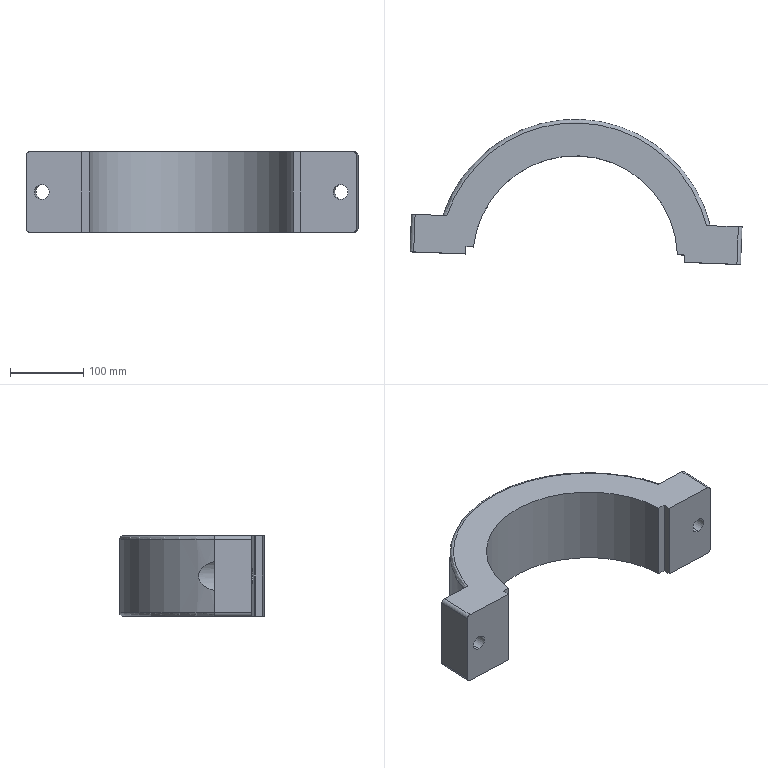Part | SolidWorks | features BaseBody 1 | 1 solid | 26 faces | box 454.449 x 198.703 x 110 mm | volume 3221578 mm3 | plane 12 | cylinder 12 | torus 2 | commonest cylinder face diameters 10 x4 20 x4 60 x2 280 x1 380 x1
STEP:
#1=CARTESIAN_POINT('',(121.261,1068.497,205.107));
#2=VERTEX_POINT('',#1);
#3=CARTESIAN_POINT('',(121.261,1068.497,315.107));
#4=VERTEX_POINT('',#3);
#5=CARTESIAN_POINT('',(121.261,1068.497,315.107));
#6=DIRECTION('',(0.,0.,1.));
#7=VECTOR('',#6,1000.);
#8=LINE('',#5,#7);
#9=EDGE_CURVE('',#2,#4,#8,.T.);
#10=ORIENTED_EDGE('',*,*,#9,.T.);
#11=CARTESIAN_POINT('',(110.911,1068.895,315.107));
#12=VERTEX_POINT('',#11);
#13=CARTESIAN_POINT('',(260.936,1063.128,315.107));
#14=DIRECTION('',(-0.9993,0.03842,0.));
#15=VECTOR('',#14,1000.);
#16=LINE('',#13,#15);
#17=EDGE_CURVE('',#4,#12,#16,.T.);
#18=ORIENTED_EDGE('',*,*,#17,.T.);
#19=CARTESIAN_POINT('',(110.911,1068.895,205.107));
#20=VERTEX_POINT('',#19);
#21=CARTESIAN_POINT('',(110.911,1068.895,-875.938));
#22=DIRECTION('',(0.,0.,1.));
#23=VECTOR('',#22,1000.);
#24=LINE('',#21,#23);
#25=EDGE_CURVE('',#20,#12,#24,.T.);
#26=ORIENTED_EDGE('',*,*,#25,.F.);
#27=CARTESIAN_POINT('',(260.936,1063.128,205.107));
#28=DIRECTION('',(-0.9993,0.03842,0.));
#29=VECTOR('',#28,1000.);
#30=LINE('',#27,#29);
#31=EDGE_CURVE('',#2,#20,#30,.T.);
#32=ORIENTED_EDGE('',*,*,#31,.F.);
#33=EDGE_LOOP('',(#10,#18,#26,#32));
#34=FACE_OUTER_BOUND('',#33,.T.);
#35=CARTESIAN_POINT('',(410.689,1057.37,-875.938));
#36=DIRECTION('',(0.03842,0.9993,0.));
#37=DIRECTION('',(0.,0.,-1.));
#38=AXIS2_PLACEMENT_3D('',#35,#36,#37);
#39=PLANE('',#38);
#40=ADVANCED_FACE('',(#34),#39,.F.);
#41=CARTESIAN_POINT('',(55.968,1061.,270.107));
#42=VERTEX_POINT('',#41);
#43=CARTESIAN_POINT('',(55.968,1061.,250.107));
#44=VERTEX_POINT('',#43);
#45=CARTESIAN_POINT('',(55.968,1061.,260.107));
#46=DIRECTION('',(-0.03842,-0.9993,0.));
#47=DIRECTION('',(0.,0.,1.));
#48=AXIS2_PLACEMENT_3D('',#45,#46,#47);
#49=CIRCLE('',#48,10.);
#50=EDGE_CURVE('',#42,#44,#49,.T.);
#51=ORIENTED_EDGE('',*,*,#50,.F.);
#52=CARTESIAN_POINT('',(55.968,1061.,260.107));
#53=DIRECTION('',(-0.03842,-0.9993,0.));
#54=DIRECTION('',(0.,0.,1.));
#55=AXIS2_PLACEMENT_3D('',#52,#53,#54);
#56=CIRCLE('',#55,10.);
#57=EDGE_CURVE('',#44,#42,#56,.T.);
#58=ORIENTED_EDGE('',*,*,#57,.F.);
#59=EDGE_LOOP('',(#51,#58));
#60=FACE_BOUND('',#59,.T.);
#61=CARTESIAN_POINT('',(110.527,1058.903,205.107));
#62=VERTEX_POINT('',#61);
#63=CARTESIAN_POINT('',(110.527,1058.903,315.107));
#64=VERTEX_POINT('',#63);
#65=CARTESIAN_POINT('',(110.527,1058.903,-875.938));
#66=DIRECTION('',(0.,0.,1.));
#67=VECTOR('',#66,1000.);
#68=LINE('',#65,#67);
#69=EDGE_CURVE('',#62,#64,#68,.T.);
#70=ORIENTED_EDGE('',*,*,#69,.T.);
#71=CARTESIAN_POINT('',(39.31,1061.641,315.107));
#72=VERTEX_POINT('',#71);
#73=CARTESIAN_POINT('',(260.552,1053.135,315.107));
#74=DIRECTION('',(-0.9993,0.03842,0.));
#75=VECTOR('',#74,1000.);
#76=LINE('',#73,#75);
#77=EDGE_CURVE('',#64,#72,#76,.T.);
#78=ORIENTED_EDGE('',*,*,#77,.T.);
#79=CARTESIAN_POINT('',(34.314,1061.833,310.107));
#80=VERTEX_POINT('',#79);
#81=CARTESIAN_POINT('',(39.31,1061.641,310.107));
#82=DIRECTION('',(-0.03842,-0.9993,0.));
#83=DIRECTION('',(0.,0.,1.));
#84=AXIS2_PLACEMENT_3D('',#81,#82,#83);
#85=CIRCLE('',#84,5.);
#86=EDGE_CURVE('',#72,#80,#85,.T.);
#87=ORIENTED_EDGE('',*,*,#86,.T.);
#88=CARTESIAN_POINT('',(34.314,1061.833,210.107));
#89=VERTEX_POINT('',#88);
#90=CARTESIAN_POINT('',(34.314,1061.833,315.107));
#91=DIRECTION('',(0.,0.,1.));
#92=VECTOR('',#91,1000.);
#93=LINE('',#90,#92);
#94=EDGE_CURVE('',#89,#80,#93,.T.);
#95=ORIENTED_EDGE('',*,*,#94,.F.);
#96=CARTESIAN_POINT('',(39.31,1061.641,205.107));
#97=VERTEX_POINT('',#96);
#98=CARTESIAN_POINT('',(39.31,1061.641,210.107));
#99=DIRECTION('',(-0.03842,-0.9993,0.));
#100=DIRECTION('',(0.,0.,1.));
#101=AXIS2_PLACEMENT_3D('',#98,#99,#100);
#102=CIRCLE('',#101,5.);
#103=EDGE_CURVE('',#89,#97,#102,.T.);
#104=ORIENTED_EDGE('',*,*,#103,.T.);
#105=CARTESIAN_POINT('',(260.552,1053.135,205.107));
#106=DIRECTION('',(-0.9993,0.03842,0.));
#107=VECTOR('',#106,1000.);
#108=LINE('',#105,#107);
#109=EDGE_CURVE('',#62,#97,#108,.T.);
#110=ORIENTED_EDGE('',*,*,#109,.F.);
#111=EDGE_LOOP('',(#70,#78,#87,#95,#104,#110));
#112=FACE_OUTER_BOUND('',#111,.T.);
#113=CARTESIAN_POINT('',(110.527,1058.903,-875.938));
#114=DIRECTION('',(0.03842,0.9993,0.));
#115=DIRECTION('',(0.,0.,-1.));
#116=AXIS2_PLACEMENT_3D('',#113,#114,#115);
#117=PLANE('',#116);
#118=ADVANCED_FACE('',(#60,#112),#117,.F.);
#119=ORIENTED_EDGE('',*,*,#25,.T.);
#120=CARTESIAN_POINT('',(79.906,262.409,315.107));
#121=DIRECTION('',(-0.03842,-0.9993,0.));
#122=VECTOR('',#121,1000.);
#123=LINE('',#120,#122);
#124=EDGE_CURVE('',#12,#64,#123,.T.);
#125=ORIENTED_EDGE('',*,*,#124,.T.);
#126=ORIENTED_EDGE('',*,*,#69,.F.);
#127=CARTESIAN_POINT('',(79.906,262.409,205.107));
#128=DIRECTION('',(-0.03842,-0.9993,0.));
#129=VECTOR('',#128,1000.);
#130=LINE('',#127,#129);
#131=EDGE_CURVE('',#20,#62,#130,.T.);
#132=ORIENTED_EDGE('',*,*,#131,.F.);
#133=EDGE_LOOP('',(#119,#125,#126,#132));
#134=FACE_OUTER_BOUND('',#133,.T.);
#135=CARTESIAN_POINT('',(110.911,1068.895,-875.938));
#136=DIRECTION('',(-0.9993,0.03842,0.));
#137=DIRECTION('',(0.,0.,1.));
#138=AXIS2_PLACEMENT_3D('',#135,#136,#137);
#139=PLANE('',#138);
#140=ADVANCED_FACE('',(#134),#139,.F.);
#141=CARTESIAN_POINT('',(481.794,1044.629,205.107));
#142=VERTEX_POINT('',#141);
#143=CARTESIAN_POINT('',(486.791,1044.437,210.107));
#144=VERTEX_POINT('',#143);
#145=CARTESIAN_POINT('',(481.794,1044.629,210.107));
#146=DIRECTION('',(-0.03842,-0.9993,0.));
#147=DIRECTION('',(0.,0.,1.));
#148=AXIS2_PLACEMENT_3D('',#145,#146,#147);
#149=CIRCLE('',#148,5.);
#150=EDGE_CURVE('',#142,#144,#149,.T.);
#151=ORIENTED_EDGE('',*,*,#150,.F.);
#152=CARTESIAN_POINT('',(483.767,1095.943,205.107));
#153=VERTEX_POINT('',#152);
#154=CARTESIAN_POINT('',(479.822,993.316,205.107));
#155=DIRECTION('',(-0.03842,-0.9993,0.));
#156=VECTOR('',#155,1000.);
#157=LINE('',#154,#156);
#158=EDGE_CURVE('',#153,#142,#157,.T.);
#159=ORIENTED_EDGE('',*,*,#158,.F.);
#160=CARTESIAN_POINT('',(488.763,1095.751,210.107));
#161=VERTEX_POINT('',#160);
#162=CARTESIAN_POINT('',(483.767,1095.943,210.107));
#163=DIRECTION('',(0.03842,0.9993,0.));
#164=DIRECTION('',(0.,0.,-1.));
#165=AXIS2_PLACEMENT_3D('',#162,#163,#164);
#166=CIRCLE('',#165,5.);
#167=EDGE_CURVE('',#161,#153,#166,.T.);
#168=ORIENTED_EDGE('',*,*,#167,.F.);
#169=CARTESIAN_POINT('',(488.763,1095.751,210.107));
#170=DIRECTION('',(0.03842,0.9993,0.));
#171=VECTOR('',#170,1000.);
#172=LINE('',#169,#171);
#173=EDGE_CURVE('',#144,#161,#172,.T.);
#174=ORIENTED_EDGE('',*,*,#173,.F.);
#175=EDGE_LOOP('',(#151,#159,#168,#174));
#176=FACE_OUTER_BOUND('',#175,.T.);
#177=CARTESIAN_POINT('',(451.173,248.135,210.107));
#178=DIRECTION('',(0.03842,0.9993,0.));
#179=DIRECTION('',(0.,0.,-1.));
#180=AXIS2_PLACEMENT_3D('',#177,#178,#179);
#181=CYLINDRICAL_SURFACE('',#180,5.);
#182=ADVANCED_FACE('',(#176),#181,.T.);
#183=ORIENTED_EDGE('',*,*,#103,.F.);
#184=CARTESIAN_POINT('',(36.287,1113.146,210.107));
#185=VERTEX_POINT('',#184);
#186=CARTESIAN_POINT('',(3.693,265.339,210.107));
#187=DIRECTION('',(-0.03842,-0.9993,0.));
#188=VECTOR('',#187,1000.);
#189=LINE('',#186,#188);
#190=EDGE_CURVE('',#185,#89,#189,.T.);
#191=ORIENTED_EDGE('',*,*,#190,.F.);
#192=CARTESIAN_POINT('',(41.283,1112.954,205.107));
#193=VERTEX_POINT('',#192);
#194=CARTESIAN_POINT('',(41.283,1112.954,210.107));
#195=DIRECTION('',(0.03842,0.9993,0.));
#196=DIRECTION('',(0.,0.,1.));
#197=AXIS2_PLACEMENT_3D('',#194,#195,#196);
#198=CIRCLE('',#197,5.);
#199=EDGE_CURVE('',#193,#185,#198,.T.);
#200=ORIENTED_EDGE('',*,*,#199,.F.);
#201=CARTESIAN_POINT('',(8.689,265.147,205.107));
#202=DIRECTION('',(0.03842,0.9993,0.));
#203=VECTOR('',#202,1000.);
#204=LINE('',#201,#203);
#205=EDGE_CURVE('',#97,#193,#204,.T.);
#206=ORIENTED_EDGE('',*,*,#205,.F.);
#207=EDGE_LOOP('',(#183,#191,#200,#206));
#208=FACE_OUTER_BOUND('',#207,.T.);
#209=CARTESIAN_POINT('',(8.689,265.147,210.107));
#210=DIRECTION('',(-0.03842,-0.9993,0.));
#211=DIRECTION('',(0.,0.,1.));
#212=AXIS2_PLACEMENT_3D('',#209,#210,#211);
#213=CYLINDRICAL_SURFACE('',#212,5.);
#214=ADVANCED_FACE('',(#208),#213,.T.);
#215=CARTESIAN_POINT('',(439.988,1097.626,205.107));
#216=VERTEX_POINT('',#215);
#217=CARTESIAN_POINT('',(445.183,1097.426,210.107));
#218=VERTEX_POINT('',#217);
#219=CARTESIAN_POINT('',(439.988,1097.626,205.107));
#220=CARTESIAN_POINT('',(440.322,1097.613,205.107));
#221=CARTESIAN_POINT('',(440.652,1097.6,205.137));
#222=CARTESIAN_POINT('',(441.311,1097.575,205.261));
#223=CARTESIAN_POINT('',(441.632,1097.563,205.352));
#224=CARTESIAN_POINT('',(442.099,1097.545,205.535));
#225=CARTESIAN_POINT('',(442.251,1097.539,205.602));
#226=CARTESIAN_POINT('',(442.547,1097.528,205.752));
#227=CARTESIAN_POINT('',(442.69,1097.522,205.832));
#228=CARTESIAN_POINT('',(443.117,1097.506,206.101));
#229=CARTESIAN_POINT('',(443.381,1097.495,206.306));
#230=CARTESIAN_POINT('',(443.746,1097.481,206.65));
#231=CARTESIAN_POINT('',(443.861,1097.477,206.769));
#232=CARTESIAN_POINT('',(444.079,1097.469,207.02));
#233=CARTESIAN_POINT('',(444.18,1097.465,207.148));
#234=CARTESIAN_POINT('',(444.472,1097.454,207.56));
#235=CARTESIAN_POINT('',(444.637,1097.447,207.85));
#236=CARTESIAN_POINT('',(444.839,1097.439,208.31));
#237=CARTESIAN_POINT('',(444.898,1097.437,208.465));
#238=CARTESIAN_POINT('',(445.,1097.433,208.782));
#239=CARTESIAN_POINT('',(445.043,1097.432,208.941));
#240=CARTESIAN_POINT('',(445.148,1097.428,209.436));
#241=CARTESIAN_POINT('',(445.183,1097.426,209.769));
#242=CARTESIAN_POINT('',(445.183,1097.426,210.107));
#243=B_SPLINE_CURVE_WITH_KNOTS('',3,(#219,#220,#221,#222,#223,#224,#225,#226,#227,#228,#229,#230,#231,#232,#233,#234,#235,#236,#237,#238,#239,#240,#241,#242),.UNSPECIFIED.,.F.,.F.,(4,2,2,2,2,2,2,2,2,2,2,4),(0.,0.125,0.25,0.3125,0.375,0.5,0.5625,0.625,0.75,0.8125,0.875,1.),.UNSPECIFIED.);
#244=EDGE_CURVE('',#216,#218,#243,.T.);
#245=ORIENTED_EDGE('',*,*,#244,.F.);
#246=CARTESIAN_POINT('',(84.79,1111.281,205.107));
#247=VERTEX_POINT('',#246);
#248=CARTESIAN_POINT('',(260.416,1053.14,205.107));
#249=DIRECTION('',(0.,0.,-1.));
#250=DIRECTION('',(0.9993,-0.03842,0.));
#251=AXIS2_PLACEMENT_3D('',#248,#249,#250);
#252=CIRCLE('',#251,185.);
#253=EDGE_CURVE('',#247,#216,#252,.T.);
#254=ORIENTED_EDGE('',*,*,#253,.F.);
#255=CARTESIAN_POINT('',(79.595,1111.481,210.107));
#256=VERTEX_POINT('',#255);
#257=CARTESIAN_POINT('',(79.595,1111.481,210.107));
#258=CARTESIAN_POINT('',(79.595,1111.481,209.773));
#259=CARTESIAN_POINT('',(79.629,1111.48,209.441));
#260=CARTESIAN_POINT('',(79.732,1111.476,208.95));
#261=CARTESIAN_POINT('',(79.775,1111.474,208.789));
#262=CARTESIAN_POINT('',(79.877,1111.47,208.471));
#263=CARTESIAN_POINT('',(79.937,1111.468,208.313));
#264=CARTESIAN_POINT('',(80.137,1111.46,207.856));
#265=CARTESIAN_POINT('',(80.302,1111.454,207.566));
#266=CARTESIAN_POINT('',(80.59,1111.443,207.157));
#267=CARTESIAN_POINT('',(80.693,1111.439,207.026));
#268=CARTESIAN_POINT('',(80.912,1111.431,206.774));
#269=CARTESIAN_POINT('',(81.029,1111.426,206.652));
#270=CARTESIAN_POINT('',(81.271,1111.417,206.423));
#271=CARTESIAN_POINT('',(81.398,1111.412,206.315));
#272=CARTESIAN_POINT('',(81.661,1111.402,206.111));
#273=CARTESIAN_POINT('',(81.799,1111.396,206.014));
#274=CARTESIAN_POINT('',(82.221,1111.38,205.748));
#275=CARTESIAN_POINT('',(82.519,1111.369,205.597));
#276=CARTESIAN_POINT('',(83.141,1111.345,205.354));
#277=CARTESIAN_POINT('',(83.463,1111.332,205.261));
#278=CARTESIAN_POINT('',(84.121,1111.307,205.138));
#279=CARTESIAN_POINT('',(84.454,1111.294,205.107));
#280=CARTESIAN_POINT('',(84.79,1111.281,205.107));
#281=B_SPLINE_CURVE_WITH_KNOTS('',3,(#257,#258,#259,#260,#261,#262,#263,#264,#265,#266,#267,#268,#269,#270,#271,#272,#273,#274,#275,#276,#277,#278,#279,#280),.UNSPECIFIED.,.F.,.F.,(4,2,2,2,2,2,2,2,2,2,2,4),(0.,0.125,0.1875,0.25,0.375,0.4375,0.5,0.5625,0.625,0.75,0.875,1.),.UNSPECIFIED.);
#282=EDGE_CURVE('',#256,#247,#281,.T.);
#283=ORIENTED_EDGE('',*,*,#282,.F.);
#284=CARTESIAN_POINT('',(260.416,1053.14,210.107));
#285=DIRECTION('',(0.,0.,1.));
#286=DIRECTION('',(0.9993,-0.03842,0.));
#287=AXIS2_PLACEMENT_3D('',#284,#285,#286);
#288=CIRCLE('',#287,190.);
#289=EDGE_CURVE('',#218,#256,#288,.T.);
#290=ORIENTED_EDGE('',*,*,#289,.F.);
#291=EDGE_LOOP('',(#245,#254,#283,#290));
#292=FACE_OUTER_BOUND('',#291,.T.);
#293=CARTESIAN_POINT('',(260.416,1053.14,210.107));
#294=DIRECTION('',(0.,0.,1.));
#295=DIRECTION('',(-0.9993,0.03842,0.));
#296=AXIS2_PLACEMENT_3D('',#293,#294,#295);
#297=TOROIDAL_SURFACE('',#296,185.,5.);
#298=ADVANCED_FACE('',(#292),#297,.T.);
#299=CARTESIAN_POINT('',(486.791,1044.437,310.107));
#300=VERTEX_POINT('',#299);
#301=CARTESIAN_POINT('',(481.794,1044.629,315.107));
#302=VERTEX_POINT('',#301);
#303=CARTESIAN_POINT('',(481.794,1044.629,310.107));
#304=DIRECTION('',(-0.03842,-0.9993,0.));
#305=DIRECTION('',(0.,0.,1.));
#306=AXIS2_PLACEMENT_3D('',#303,#304,#305);
#307=CIRCLE('',#306,5.);
#308=EDGE_CURVE('',#300,#302,#307,.T.);
#309=ORIENTED_EDGE('',*,*,#308,.F.);
#310=CARTESIAN_POINT('',(488.763,1095.751,310.107));
#311=VERTEX_POINT('',#310);
#312=CARTESIAN_POINT('',(456.17,247.943,310.107));
#313=DIRECTION('',(-0.03842,-0.9993,0.));
#314=VECTOR('',#313,1000.);
#315=LINE('',#312,#314);
#316=EDGE_CURVE('',#311,#300,#315,.T.);
#317=ORIENTED_EDGE('',*,*,#316,.F.);
#318=CARTESIAN_POINT('',(483.767,1095.943,315.107));
#319=VERTEX_POINT('',#318);
#320=CARTESIAN_POINT('',(483.767,1095.943,310.107));
#321=DIRECTION('',(0.03842,0.9993,0.));
#322=DIRECTION('',(0.,0.,-1.));
#323=AXIS2_PLACEMENT_3D('',#320,#321,#322);
#324=CIRCLE('',#323,5.);
#325=EDGE_CURVE('',#319,#311,#324,.T.);
#326=ORIENTED_EDGE('',*,*,#325,.F.);
#327=CARTESIAN_POINT('',(451.173,248.135,315.107));
#328=DIRECTION('',(0.03842,0.9993,0.));
#329=VECTOR('',#328,1000.);
#330=LINE('',#327,#329);
#331=EDGE_CURVE('',#302,#319,#330,.T.);
#332=ORIENTED_EDGE('',*,*,#331,.F.);
#333=EDGE_LOOP('',(#309,#317,#326,#332));
#334=FACE_OUTER_BOUND('',#333,.T.);
#335=CARTESIAN_POINT('',(451.173,248.135,310.107));
#336=DIRECTION('',(-0.03842,-0.9993,0.));
#337=DIRECTION('',(0.,0.,1.));
#338=AXIS2_PLACEMENT_3D('',#335,#336,#337);
#339=CYLINDRICAL_SURFACE('',#338,5.);
#340=ADVANCED_FACE('',(#334),#339,.T.);
#341=CARTESIAN_POINT('',(445.183,1097.426,310.107));
#342=VERTEX_POINT('',#341);
#343=CARTESIAN_POINT('',(439.988,1097.626,315.107));
#344=VERTEX_POINT('',#343);
#345=CARTESIAN_POINT('',(445.183,1097.426,310.107));
#346=CARTESIAN_POINT('',(445.183,1097.426,310.441));
#347=CARTESIAN_POINT('',(445.148,1097.428,310.772));
#348=CARTESIAN_POINT('',(445.045,1097.432,311.263));
#349=CARTESIAN_POINT('',(445.002,1097.433,311.424));
#350=CARTESIAN_POINT('',(444.9,1097.437,311.742));
#351=CARTESIAN_POINT('',(444.84,1097.439,311.901));
#352=CARTESIAN_POINT('',(444.64,1097.447,312.357));
#353=CARTESIAN_POINT('',(444.476,1097.453,312.648));
#354=CARTESIAN_POINT('',(444.187,1097.465,313.056));
#355=CARTESIAN_POINT('',(444.084,1097.468,313.188));
#356=CARTESIAN_POINT('',(443.865,1097.477,313.439));
#357=CARTESIAN_POINT('',(443.748,1097.481,313.562));
#358=CARTESIAN_POINT('',(443.506,1097.491,313.79));
#359=CARTESIAN_POINT('',(443.38,1097.496,313.898));
#360=CARTESIAN_POINT('',(443.116,1097.506,314.103));
#361=CARTESIAN_POINT('',(442.978,1097.511,314.199));
#362=CARTESIAN_POINT('',(442.556,1097.527,314.466));
#363=CARTESIAN_POINT('',(442.258,1097.539,314.616));
#364=CARTESIAN_POINT('',(441.636,1097.563,314.86));
#365=CARTESIAN_POINT('',(441.314,1097.575,314.952));
#366=CARTESIAN_POINT('',(440.656,1097.6,315.076));
#367=CARTESIAN_POINT('',(440.323,1097.613,315.107));
#368=CARTESIAN_POINT('',(439.988,1097.626,315.107));
#369=B_SPLINE_CURVE_WITH_KNOTS('',3,(#345,#346,#347,#348,#349,#350,#351,#352,#353,#354,#355,#356,#357,#358,#359,#360,#361,#362,#363,#364,#365,#366,#367,#368),.UNSPECIFIED.,.F.,.F.,(4,2,2,2,2,2,2,2,2,2,2,4),(0.,0.125,0.1875,0.25,0.375,0.4375,0.5,0.5625,0.625,0.75,0.875,1.),.UNSPECIFIED.);
#370=EDGE_CURVE('',#342,#344,#369,.T.);
#371=ORIENTED_EDGE('',*,*,#370,.F.);
#372=CARTESIAN_POINT('',(79.595,1111.481,310.107));
#373=VERTEX_POINT('',#372);
#374=CARTESIAN_POINT('',(260.416,1053.14,310.107));
#375=DIRECTION('',(0.,0.,-1.));
#376=DIRECTION('',(0.9993,-0.03842,0.));
#377=AXIS2_PLACEMENT_3D('',#374,#375,#376);
#378=CIRCLE('',#377,190.);
#379=EDGE_CURVE('',#373,#342,#378,.T.);
#380=ORIENTED_EDGE('',*,*,#379,.F.);
#381=CARTESIAN_POINT('',(84.79,1111.281,315.107));
#382=VERTEX_POINT('',#381);
#383=CARTESIAN_POINT('',(84.79,1111.281,315.107));
#384=CARTESIAN_POINT('',(84.455,1111.294,315.107));
#385=CARTESIAN_POINT('',(84.125,1111.307,315.076));
#386=CARTESIAN_POINT('',(83.466,1111.332,314.953));
#387=CARTESIAN_POINT('',(83.145,1111.345,314.861));
#388=CARTESIAN_POINT('',(82.679,1111.363,314.679));
#389=CARTESIAN_POINT('',(82.527,1111.368,314.611));
#390=CARTESIAN_POINT('',(82.23,1111.38,314.462));
#391=CARTESIAN_POINT('',(82.087,1111.385,314.381));
#392=CARTESIAN_POINT('',(81.66,1111.402,314.112));
#393=CARTESIAN_POINT('',(81.396,1111.412,313.908));
#394=CARTESIAN_POINT('',(81.031,1111.426,313.564));
#395=CARTESIAN_POINT('',(80.916,1111.43,313.444));
#396=CARTESIAN_POINT('',(80.699,1111.439,313.194));
#397=CARTESIAN_POINT('',(80.597,1111.443,313.065));
#398=CARTESIAN_POINT('',(80.305,1111.454,312.654));
#399=CARTESIAN_POINT('',(80.14,1111.46,312.363));
#400=CARTESIAN_POINT('',(79.938,1111.468,311.904));
#401=CARTESIAN_POINT('',(79.879,1111.47,311.748));
#402=CARTESIAN_POINT('',(79.777,1111.474,311.432));
#403=CARTESIAN_POINT('',(79.735,1111.476,311.273));
#404=CARTESIAN_POINT('',(79.63,1111.48,310.778));
#405=CARTESIAN_POINT('',(79.595,1111.481,310.444));
#406=CARTESIAN_POINT('',(79.595,1111.481,310.107));
#407=B_SPLINE_CURVE_WITH_KNOTS('',3,(#383,#384,#385,#386,#387,#388,#389,#390,#391,#392,#393,#394,#395,#396,#397,#398,#399,#400,#401,#402,#403,#404,#405,#406),.UNSPECIFIED.,.F.,.F.,(4,2,2,2,2,2,2,2,2,2,2,4),(0.,0.125,0.25,0.3125,0.375,0.5,0.5625,0.625,0.75,0.8125,0.875,1.),.UNSPECIFIED.);
#408=EDGE_CURVE('',#382,#373,#407,.T.);
#409=ORIENTED_EDGE('',*,*,#408,.F.);
#410=CARTESIAN_POINT('',(260.416,1053.14,315.107));
#411=DIRECTION('',(0.,0.,1.));
#412=DIRECTION('',(0.9993,-0.03842,0.));
#413=AXIS2_PLACEMENT_3D('',#410,#411,#412);
#414=CIRCLE('',#413,185.);
#415=EDGE_CURVE('',#344,#382,#414,.T.);
#416=ORIENTED_EDGE('',*,*,#415,.F.);
#417=EDGE_LOOP('',(#371,#380,#409,#416));
#418=FACE_OUTER_BOUND('',#417,.T.);
#419=CARTESIAN_POINT('',(260.416,1053.14,310.107));
#420=DIRECTION('',(0.,0.,1.));
#421=DIRECTION('',(-0.9993,0.03842,0.));
#422=AXIS2_PLACEMENT_3D('',#419,#420,#421);
#423=TOROIDAL_SURFACE('',#422,185.,5.);
#424=ADVANCED_FACE('',(#418),#423,.T.);
#425=ORIENTED_EDGE('',*,*,#86,.F.);
#426=CARTESIAN_POINT('',(41.283,1112.954,315.107));
#427=VERTEX_POINT('',#426);
#428=CARTESIAN_POINT('',(37.301,1009.365,315.107));
#429=DIRECTION('',(-0.03842,-0.9993,0.));
#430=VECTOR('',#429,1000.);
#431=LINE('',#428,#430);
#432=EDGE_CURVE('',#427,#72,#431,.T.);
#433=ORIENTED_EDGE('',*,*,#432,.F.);
#434=CARTESIAN_POINT('',(36.287,1113.146,310.107));
#435=VERTEX_POINT('',#434);
#436=CARTESIAN_POINT('',(41.283,1112.954,310.107));
#437=DIRECTION('',(0.03842,0.9993,0.));
#438=DIRECTION('',(0.,0.,1.));
#439=AXIS2_PLACEMENT_3D('',#436,#437,#438);
#440=CIRCLE('',#439,5.);
#441=EDGE_CURVE('',#435,#427,#440,.T.);
#442=ORIENTED_EDGE('',*,*,#441,.F.);
#443=CARTESIAN_POINT('',(36.287,1113.146,310.107));
#444=DIRECTION('',(0.03842,0.9993,0.));
#445=VECTOR('',#444,1000.);
#446=LINE('',#443,#445);
#447=EDGE_CURVE('',#80,#435,#446,.T.);
#448=ORIENTED_EDGE('',*,*,#447,.F.);
#449=EDGE_LOOP('',(#425,#433,#442,#448));
#450=FACE_OUTER_BOUND('',#449,.T.);
#451=CARTESIAN_POINT('',(8.689,265.147,310.107));
#452=DIRECTION('',(0.03842,0.9993,0.));
#453=DIRECTION('',(0.,0.,-1.));
#454=AXIS2_PLACEMENT_3D('',#451,#452,#453);
#455=CYLINDRICAL_SURFACE('',#454,5.);
#456=ADVANCED_FACE('',(#450),#455,.T.);
#457=CARTESIAN_POINT('',(79.595,1111.481,280.853));
#458=VERTEX_POINT('',#457);
#459=CARTESIAN_POINT('',(79.595,1111.481,239.36));
#460=VERTEX_POINT('',#459);
#461=CARTESIAN_POINT('',(79.595,1111.481,280.853));
#462=CARTESIAN_POINT('',(80.041,1112.865,280.443));
#463=CARTESIAN_POINT('',(80.487,1114.194,280.007));
#464=CARTESIAN_POINT('',(81.152,1116.108,279.312));
#465=CARTESIAN_POINT('',(81.373,1116.733,279.074));
#466=CARTESIAN_POINT('',(81.702,1117.65,278.707));
#467=CARTESIAN_POINT('',(81.866,1118.103,278.52));
#468=CARTESIAN_POINT('',(82.056,1118.623,278.298));
#469=CARTESIAN_POINT('',(82.151,1118.881,278.186));
#470=CARTESIAN_POINT('',(82.199,1119.009,278.129));
#471=CARTESIAN_POINT('',(82.223,1119.073,278.101));
#472=CARTESIAN_POINT('',(82.233,1119.1,278.089));
#473=CARTESIAN_POINT('',(82.239,1119.119,278.081));
#474=CARTESIAN_POINT('',(82.242,1119.127,278.077));
#475=CARTESIAN_POINT('',(82.741,1120.472,277.481));
#476=CARTESIAN_POINT('',(83.222,1121.726,276.856));
#477=CARTESIAN_POINT('',(83.917,1123.486,275.87));
#478=CARTESIAN_POINT('',(84.144,1124.052,275.533));
#479=CARTESIAN_POINT('',(84.477,1124.872,275.016));
#480=CARTESIAN_POINT('',(84.641,1125.275,274.754));
#481=CARTESIAN_POINT('',(84.829,1125.731,274.443));
#482=CARTESIAN_POINT('',(84.923,1125.956,274.286));
#483=CARTESIAN_POINT('',(84.969,1126.067,274.207));
#484=CARTESIAN_POINT('',(84.992,1126.123,274.167));
#485=CARTESIAN_POINT('',(85.004,1126.151,274.148));
#486=CARTESIAN_POINT('',(85.008,1126.163,274.139));
#487=CARTESIAN_POINT('',(85.012,1126.17,274.134));
#488=CARTESIAN_POINT('',(85.013,1126.173,274.131));
#489=CARTESIAN_POINT('',(85.532,1127.419,273.242));
#490=CARTESIAN_POINT('',(86.007,1128.526,272.315));
#491=CARTESIAN_POINT('',(86.649,1129.988,270.868));
#492=CARTESIAN_POINT('',(86.851,1130.442,270.376));
#493=CARTESIAN_POINT('',(87.134,1131.073,269.625));
#494=CARTESIAN_POINT('',(87.271,1131.377,269.246));
#495=CARTESIAN_POINT('',(87.422,1131.709,268.798));
#496=CARTESIAN_POINT('',(87.495,1131.869,268.572));
#497=CARTESIAN_POINT('',(87.531,1131.948,268.459));
#498=CARTESIAN_POINT('',(87.549,1131.988,268.402));
#499=CARTESIAN_POINT('',(87.556,1132.004,268.378));
#500=CARTESIAN_POINT('',(87.561,1132.015,268.362));
#501=CARTESIAN_POINT('',(87.563,1132.02,268.355));
#502=CARTESIAN_POINT('',(87.758,1132.447,267.73));
#503=CARTESIAN_POINT('',(87.93,1132.819,267.105));
#504=CARTESIAN_POINT('',(88.155,1133.304,266.156));
#505=CARTESIAN_POINT('',(88.259,1133.528,265.679));
#506=CARTESIAN_POINT('',(88.366,1133.757,265.117));
#507=CARTESIAN_POINT('',(88.416,1133.863,264.834));
#508=CARTESIAN_POINT('',(88.44,1133.914,264.693));
#509=CARTESIAN_POINT('',(88.45,1133.936,264.632));
#510=CARTESIAN_POINT('',(88.457,1133.95,264.592));
#511=CARTESIAN_POINT('',(88.46,1133.956,264.573));
#512=CARTESIAN_POINT('',(88.579,1134.208,263.848));
#513=CARTESIAN_POINT('',(88.666,1134.394,263.14));
#514=CARTESIAN_POINT('',(88.757,1134.584,262.071));
#515=CARTESIAN_POINT('',(88.78,1134.633,261.715));
#516=CARTESIAN_POINT('',(88.812,1134.702,260.999));
#517=CARTESIAN_POINT('',(88.822,1134.721,260.643));
#518=CARTESIAN_POINT('',(88.829,1134.736,259.562));
#519=CARTESIAN_POINT('',(88.805,1134.686,258.843));
#520=CARTESIAN_POINT('',(88.728,1134.523,257.769));
#521=CARTESIAN_POINT('',(88.678,1134.419,257.233));
#522=CARTESIAN_POINT('',(88.603,1134.259,256.61));
#523=CARTESIAN_POINT('',(88.561,1134.17,256.3));
#524=CARTESIAN_POINT('',(88.538,1134.122,256.144));
#525=CARTESIAN_POINT('',(88.529,1134.102,256.078));
#526=CARTESIAN_POINT('',(88.522,1134.088,256.034));
#527=CARTESIAN_POINT('',(88.518,1134.08,256.01));
#528=CARTESIAN_POINT('',(88.416,1133.863,255.334));
#529=CARTESIAN_POINT('',(88.294,1133.603,254.684));
#530=CARTESIAN_POINT('',(88.077,1133.137,253.722));
#531=CARTESIAN_POINT('',(87.961,1132.886,253.244));
#532=CARTESIAN_POINT('',(87.81,1132.559,252.692));
#533=CARTESIAN_POINT('',(87.732,1132.388,252.417));
#534=CARTESIAN_POINT('',(87.691,1132.3,252.28));
#535=CARTESIAN_POINT('',(87.671,1132.256,252.211));
#536=CARTESIAN_POINT('',(87.662,1132.237,252.182));
#537=CARTESIAN_POINT('',(87.657,1132.224,252.163));
#538=CARTESIAN_POINT('',(87.653,1132.216,252.151));
#539=CARTESIAN_POINT('',(87.333,1131.516,251.086));
#540=CARTESIAN_POINT('',(86.956,1130.684,250.063));
#541=CARTESIAN_POINT('',(86.316,1129.231,248.586));
#542=CARTESIAN_POINT('',(86.09,1128.712,248.103));
#543=CARTESIAN_POINT('',(85.734,1127.883,247.395));
#544=CARTESIAN_POINT('',(85.552,1127.455,247.044));
#545=CARTESIAN_POINT('',(85.331,1126.934,246.641));
#546=CARTESIAN_POINT('',(85.22,1126.668,246.442));
#547=CARTESIAN_POINT('',(85.163,1126.533,246.343));
#548=CARTESIAN_POINT('',(85.135,1126.465,246.293));
#549=CARTESIAN_POINT('',(85.123,1126.436,246.272));
#550=CARTESIAN_POINT('',(85.115,1126.417,246.258));
#551=CARTESIAN_POINT('',(85.11,1126.405,246.249));
#552=CARTESIAN_POINT('',(84.679,1125.374,245.499));
#553=CARTESIAN_POINT('',(84.226,1124.266,244.789));
#554=CARTESIAN_POINT('',(83.518,1122.478,243.775));
#555=CARTESIAN_POINT('',(83.278,1121.861,243.446));
#556=CARTESIAN_POINT('',(82.91,1120.904,242.965));
#557=CARTESIAN_POINT('',(82.725,1120.417,242.728));
#558=CARTESIAN_POINT('',(82.506,1119.835,242.456));
#559=CARTESIAN_POINT('',(82.396,1119.541,242.322));
#560=CARTESIAN_POINT('',(82.341,1119.393,242.255));
#561=CARTESIAN_POINT('',(82.314,1119.319,242.222));
#562=CARTESIAN_POINT('',(82.302,1119.287,242.207));
#563=CARTESIAN_POINT('',(82.294,1119.266,242.198));
#564=CARTESIAN_POINT('',(82.289,1119.254,242.193));
#565=CARTESIAN_POINT('',(81.408,1116.879,241.132));
#566=CARTESIAN_POINT('',(80.501,1114.291,240.194));
#567=CARTESIAN_POINT('',(79.595,1111.481,239.36));
#568=B_SPLINE_CURVE_WITH_KNOTS('',3,(#461,#462,#463,#464,#465,#466,#467,#468,#469,#470,#471,#472,#473,#474,#475,#476,#477,#478,#479,#480,#481,#482,#483,#484,#485,#486,#487,#488,#489,#490,#491,#492,#493,#494,#495,#496,#497,#498,#499,#500,#501,#502,#503,#504,#505,#506,#507,#508,#509,#510,#511,#512,#513,#514,#515,#516,#517,#518,#519,#520,#521,#522,#523,#524,#525,#526,#527,#528,#529,#530,#531,#532,#533,#534,#535,#536,#537,#538,#539,#540,#541,#542,#543,#544,#545,#546,#547,#548,#549,#550,#551,#552,#553,#554,#555,#556,#557,#558,#559,#560,#561,#562,#563,#564,#565,#566,#567),.UNSPECIFIED.,.F.,.F.,(4,2,2,1,1,1,1,1,2,2,2,2,1,1,1,1,1,1,2,2,2,2,1,1,1,1,1,2,2,2,1,1,1,1,2,2,2,2,2,2,1,1,1,1,2,2,2,1,1,1,1,1,2,2,2,2,1,1,1,1,1,2,2,2,2,1,1,1,1,1,2,2,4),(0.,0.0625,0.09375,0.1094,0.1172,0.1211,0.123,0.124,0.1245,0.125,0.1875,0.2188,0.2344,0.2422,0.2461,0.248,0.249,0.2495,0.2498,0.25,0.3125,0.3438,0.3594,0.3672,0.3711,0.373,0.374,0.3745,0.375,0.4063,0.4219,0.4297,0.4336,0.4355,0.4365,0.4375,0.4688,0.4844,0.5,0.5313,0.5469,0.5547,0.5586,0.5605,0.5615,0.5625,0.5938,0.6094,0.6172,0.6211,0.623,0.624,0.6245,0.625,0.6875,0.7188,0.7344,0.7422,0.7461,0.748,0.749,0.7495,0.75,0.8125,0.8438,0.8594,0.8672,0.8711,0.873,0.874,0.8745,0.875,1.),.UNSPECIFIED.);
#569=EDGE_CURVE('',#458,#460,#568,.T.);
#570=ORIENTED_EDGE('',*,*,#569,.T.);
#571=CARTESIAN_POINT('',(57.941,1112.314,260.107));
#572=DIRECTION('',(0.03842,0.9993,0.));
#573=DIRECTION('',(0.,0.,1.));
#574=AXIS2_PLACEMENT_3D('',#571,#572,#573);
#575=CIRCLE('',#574,30.);
#576=EDGE_CURVE('',#458,#460,#575,.T.);
#577=ORIENTED_EDGE('',*,*,#576,.F.);
#578=EDGE_LOOP('',(#570,#577));
#579=FACE_OUTER_BOUND('',#578,.T.);
#580=CARTESIAN_POINT('',(61.782,1212.24,260.107));
#581=DIRECTION('',(-0.03842,-0.9993,0.));
#582=DIRECTION('',(0.,0.,1.));
#583=AXIS2_PLACEMENT_3D('',#580,#581,#582);
#584=CYLINDRICAL_SURFACE('',#583,30.);
#585=ADVANCED_FACE('',(#579),#584,.F.);
#586=CARTESIAN_POINT('',(445.183,1097.426,280.853));
#587=VERTEX_POINT('',#586);
#588=CARTESIAN_POINT('',(445.183,1097.426,239.36));
#589=VERTEX_POINT('',#588);
#590=CARTESIAN_POINT('',(466.837,1096.594,260.107));
#591=DIRECTION('',(-0.03842,-0.9993,0.));
#592=DIRECTION('',(0.,0.,1.));
#593=AXIS2_PLACEMENT_3D('',#590,#591,#592);
#594=CIRCLE('',#593,30.);
#595=EDGE_CURVE('',#587,#589,#594,.T.);
#596=ORIENTED_EDGE('',*,*,#595,.T.);
#597=CARTESIAN_POINT('',(445.183,1097.426,280.853));
#598=CARTESIAN_POINT('',(444.84,1098.857,280.438));
#599=CARTESIAN_POINT('',(444.494,1100.225,279.998));
#600=CARTESIAN_POINT('',(443.978,1102.184,279.303));
#601=CARTESIAN_POINT('',(443.807,1102.821,279.066));
#602=CARTESIAN_POINT('',(443.551,1103.754,278.7));
#603=CARTESIAN_POINT('',(443.423,1104.215,278.515));
#604=CARTESIAN_POINT('',(443.274,1104.742,278.295));
#605=CARTESIAN_POINT('',(443.2,1105.004,278.184));
#606=CARTESIAN_POINT('',(443.164,1105.133,278.129));
#607=CARTESIAN_POINT('',(443.145,1105.198,278.101));
#608=CARTESIAN_POINT('',(443.137,1105.226,278.089));
#609=CARTESIAN_POINT('',(443.132,1105.245,278.081));
#610=CARTESIAN_POINT('',(443.13,1105.252,278.077));
#611=CARTESIAN_POINT('',(442.734,1106.639,277.477));
#612=CARTESIAN_POINT('',(442.349,1107.929,276.851));
#613=CARTESIAN_POINT('',(441.792,1109.737,275.865));
#614=CARTESIAN_POINT('',(441.609,1110.318,275.528));
#615=CARTESIAN_POINT('',(441.341,1111.159,275.012));
#616=CARTESIAN_POINT('',(441.209,1111.571,274.751));
#617=CARTESIAN_POINT('',(441.057,1112.038,274.441));
#618=CARTESIAN_POINT('',(440.981,1112.268,274.285));
#619=CARTESIAN_POINT('',(440.944,1112.383,274.206));
#620=CARTESIAN_POINT('',(440.925,1112.439,274.167));
#621=CARTESIAN_POINT('',(440.916,1112.468,274.148));
#622=CARTESIAN_POINT('',(440.912,1112.48,274.139));
#623=CARTESIAN_POINT('',(440.909,1112.488,274.134));
#624=CARTESIAN_POINT('',(440.908,1112.491,274.131));
#625=CARTESIAN_POINT('',(440.486,1113.773,273.241));
#626=CARTESIAN_POINT('',(440.097,1114.913,272.316));
#627=CARTESIAN_POINT('',(439.57,1116.418,270.87));
#628=CARTESIAN_POINT('',(439.404,1116.886,270.379));
#629=CARTESIAN_POINT('',(439.17,1117.538,269.627));
#630=CARTESIAN_POINT('',(439.057,1117.851,269.248));
#631=CARTESIAN_POINT('',(438.932,1118.194,268.799));
#632=CARTESIAN_POINT('',(438.871,1118.36,268.573));
#633=CARTESIAN_POINT('',(438.841,1118.442,268.459));
#634=CARTESIAN_POINT('',(438.827,1118.483,268.403));
#635=CARTESIAN_POINT('',(438.82,1118.5,268.378));
#636=CARTESIAN_POINT('',(438.816,1118.511,268.362));
#637=CARTESIAN_POINT('',(438.814,1118.516,268.355));
#638=CARTESIAN_POINT('',(438.653,1118.957,267.73));
#639=CARTESIAN_POINT('',(438.51,1119.341,267.107));
#640=CARTESIAN_POINT('',(438.323,1119.841,266.158));
#641=CARTESIAN_POINT('',(438.265,1119.995,265.84));
#642=CARTESIAN_POINT('',(438.185,1120.207,265.359));
#643=CARTESIAN_POINT('',(438.147,1120.309,265.118));
#644=CARTESIAN_POINT('',(438.105,1120.419,264.835));
#645=CARTESIAN_POINT('',(438.085,1120.472,264.693));
#646=CARTESIAN_POINT('',(438.077,1120.494,264.633));
#647=CARTESIAN_POINT('',(438.071,1120.509,264.592));
#648=CARTESIAN_POINT('',(438.069,1120.516,264.573));
#649=CARTESIAN_POINT('',(437.97,1120.776,263.848));
#650=CARTESIAN_POINT('',(437.897,1120.968,263.14));
#651=CARTESIAN_POINT('',(437.821,1121.165,262.073));
#652=CARTESIAN_POINT('',(437.802,1121.215,261.716));
#653=CARTESIAN_POINT('',(437.775,1121.286,261.001));
#654=CARTESIAN_POINT('',(437.767,1121.306,260.643));
#655=CARTESIAN_POINT('',(437.761,1121.321,259.561));
#656=CARTESIAN_POINT('',(437.781,1121.27,258.842));
#657=CARTESIAN_POINT('',(437.846,1121.101,257.769));
#658=CARTESIAN_POINT('',(437.873,1121.03,257.412));
#659=CARTESIAN_POINT('',(437.923,1120.9,256.877));
#660=CARTESIAN_POINT('',(437.95,1120.829,256.611));
#661=CARTESIAN_POINT('',(437.985,1120.736,256.3));
#662=CARTESIAN_POINT('',(438.004,1120.687,256.145));
#663=CARTESIAN_POINT('',(438.012,1120.666,256.078));
#664=CARTESIAN_POINT('',(438.017,1120.651,256.034));
#665=CARTESIAN_POINT('',(438.02,1120.644,256.01));
#666=CARTESIAN_POINT('',(438.106,1120.419,255.332));
#667=CARTESIAN_POINT('',(438.207,1120.15,254.682));
#668=CARTESIAN_POINT('',(438.388,1119.669,253.721));
#669=CARTESIAN_POINT('',(438.452,1119.496,253.402));
#670=CARTESIAN_POINT('',(438.556,1119.217,252.928));
#671=CARTESIAN_POINT('',(438.609,1119.073,252.691));
#672=CARTESIAN_POINT('',(438.675,1118.896,252.417));
#673=CARTESIAN_POINT('',(438.708,1118.805,252.28));
#674=CARTESIAN_POINT('',(438.725,1118.76,252.211));
#675=CARTESIAN_POINT('',(438.732,1118.74,252.182));
#676=CARTESIAN_POINT('',(438.737,1118.727,252.163));
#677=CARTESIAN_POINT('',(438.74,1118.719,252.152));
#678=CARTESIAN_POINT('',(438.881,1118.334,251.584));
#679=CARTESIAN_POINT('',(439.034,1117.916,251.035));
#680=CARTESIAN_POINT('',(439.281,1117.228,250.226));
#681=CARTESIAN_POINT('',(439.409,1116.869,249.825));
#682=CARTESIAN_POINT('',(439.567,1116.425,249.364));
#683=CARTESIAN_POINT('',(439.648,1116.196,249.135));
#684=CARTESIAN_POINT('',(439.688,1116.08,249.021));
#685=CARTESIAN_POINT('',(439.709,1116.021,248.964));
#686=CARTESIAN_POINT('',(439.718,1115.996,248.94));
#687=CARTESIAN_POINT('',(439.724,1115.98,248.924));
#688=CARTESIAN_POINT('',(439.727,1115.97,248.915));
#689=CARTESIAN_POINT('',(439.897,1115.483,248.445));
#690=CARTESIAN_POINT('',(440.074,1114.974,247.991));
#691=CARTESIAN_POINT('',(440.35,1114.163,247.325));
#692=CARTESIAN_POINT('',(440.491,1113.747,246.996));
#693=CARTESIAN_POINT('',(440.66,1113.241,246.618));
#694=CARTESIAN_POINT('',(440.746,1112.983,246.43));
#695=CARTESIAN_POINT('',(440.789,1112.853,246.337));
#696=CARTESIAN_POINT('',(440.811,1112.787,246.29));
#697=CARTESIAN_POINT('',(440.82,1112.759,246.27));
#698=CARTESIAN_POINT('',(440.826,1112.74,246.257));
#699=CARTESIAN_POINT('',(440.829,1112.73,246.249));
#700=CARTESIAN_POINT('',(441.178,1111.674,245.503));
#701=CARTESIAN_POINT('',(441.543,1110.539,244.795));
#702=CARTESIAN_POINT('',(442.111,1108.702,243.781));
#703=CARTESIAN_POINT('',(442.304,1108.068,243.451));
#704=CARTESIAN_POINT('',(442.598,1107.083,242.968));
#705=CARTESIAN_POINT('',(442.746,1106.582,242.73));
#706=CARTESIAN_POINT('',(442.92,1105.982,242.458));
#707=CARTESIAN_POINT('',(443.007,1105.679,242.323));
#708=CARTESIAN_POINT('',(443.051,1105.526,242.255));
#709=CARTESIAN_POINT('',(443.073,1105.45,242.222));
#710=CARTESIAN_POINT('',(443.083,1105.417,242.208));
#711=CARTESIAN_POINT('',(443.089,1105.395,242.198));
#712=CARTESIAN_POINT('',(443.092,1105.383,242.193));
#713=CARTESIAN_POINT('',(443.78,1102.98,241.147));
#714=CARTESIAN_POINT('',(444.486,1100.333,240.204));
#715=CARTESIAN_POINT('',(445.183,1097.426,239.36));
#716=B_SPLINE_CURVE_WITH_KNOTS('',3,(#597,#598,#599,#600,#601,#602,#603,#604,#605,#606,#607,#608,#609,#610,#611,#612,#613,#614,#615,#616,#617,#618,#619,#620,#621,#622,#623,#624,#625,#626,#627,#628,#629,#630,#631,#632,#633,#634,#635,#636,#637,#638,#639,#640,#641,#642,#643,#644,#645,#646,#647,#648,#649,#650,#651,#652,#653,#654,#655,#656,#657,#658,#659,#660,#661,#662,#663,#664,#665,#666,#667,#668,#669,#670,#671,#672,#673,#674,#675,#676,#677,#678,#679,#680,#681,#682,#683,#684,#685,#686,#687,#688,#689,#690,#691,#692,#693,#694,#695,#696,#697,#698,#699,#700,#701,#702,#703,#704,#705,#706,#707,#708,#709,#710,#711,#712,#713,#714,#715),.UNSPECIFIED.,.F.,.F.,(4,2,2,1,1,1,1,1,2,2,2,2,1,1,1,1,1,1,2,2,2,2,1,1,1,1,1,2,2,2,2,1,1,1,2,2,2,2,2,2,2,1,1,1,2,2,2,2,1,1,1,1,2,2,2,1,1,1,1,1,2,2,2,1,1,1,1,1,2,2,2,2,1,1,1,1,1,2,2,4),(0.,0.0625,0.09375,0.1094,0.1172,0.1211,0.123,0.124,0.1245,0.125,0.1875,0.2187,0.2344,0.2422,0.2461,0.248,0.249,0.2495,0.2498,0.25,0.3125,0.3438,0.3594,0.3672,0.3711,0.373,0.374,0.3745,0.375,0.4063,0.4219,0.4297,0.4336,0.4355,0.4365,0.4375,0.4688,0.4844,0.5,0.5313,0.5469,0.5547,0.5586,0.5605,0.5615,0.5625,0.5938,0.6094,0.6172,0.6211,0.623,0.624,0.6245,0.625,0.6562,0.6719,0.6797,0.6836,0.6855,0.6865,0.687,0.6875,0.7187,0.7344,0.7422,0.7461,0.748,0.749,0.7495,0.75,0.8125,0.8438,0.8594,0.8672,0.8711,0.873,0.874,0.8745,0.875,1.),.UNSPECIFIED.);
#717=EDGE_CURVE('',#587,#589,#716,.T.);
#718=ORIENTED_EDGE('',*,*,#717,.F.);
#719=EDGE_LOOP('',(#596,#718));
#720=FACE_OUTER_BOUND('',#719,.T.);
#721=CARTESIAN_POINT('',(470.678,1196.52,260.107));
#722=DIRECTION('',(-0.03842,-0.9993,0.));
#723=DIRECTION('',(0.,0.,1.));
#724=AXIS2_PLACEMENT_3D('',#721,#722,#723);
#725=CYLINDRICAL_SURFACE('',#724,30.);
#726=ADVANCED_FACE('',(#720),#725,.F.);
#727=CARTESIAN_POINT('',(464.864,1045.28,250.107));
#728=VERTEX_POINT('',#727);
#729=CARTESIAN_POINT('',(466.837,1096.594,250.107));
#730=VERTEX_POINT('',#729);
#731=CARTESIAN_POINT('',(462.995,996.668,250.107));
#732=DIRECTION('',(0.03842,0.9993,0.));
#733=VECTOR('',#732,1000.);
#734=LINE('',#731,#733);
#735=EDGE_CURVE('',#728,#730,#734,.T.);
#736=ORIENTED_EDGE('',*,*,#735,.F.);
#737=CARTESIAN_POINT('',(464.864,1045.28,270.107));
#738=VERTEX_POINT('',#737);
#739=CARTESIAN_POINT('',(464.864,1045.28,260.107));
#740=DIRECTION('',(0.03842,0.9993,0.));
#741=DIRECTION('',(0.,0.,1.));
#742=AXIS2_PLACEMENT_3D('',#739,#740,#741);
#743=CIRCLE('',#742,10.);
#744=EDGE_CURVE('',#738,#728,#743,.T.);
#745=ORIENTED_EDGE('',*,*,#744,.F.);
#746=CARTESIAN_POINT('',(466.837,1096.594,270.107));
#747=VERTEX_POINT('',#746);
#748=CARTESIAN_POINT('',(462.995,996.668,270.107));
#749=DIRECTION('',(0.03842,0.9993,0.));
#750=VECTOR('',#749,1000.);
#751=LINE('',#748,#750);
#752=EDGE_CURVE('',#738,#747,#751,.T.);
#753=ORIENTED_EDGE('',*,*,#752,.T.);
#754=CARTESIAN_POINT('',(466.837,1096.594,260.107));
#755=DIRECTION('',(-0.03842,-0.9993,0.));
#756=DIRECTION('',(0.,0.,1.));
#757=AXIS2_PLACEMENT_3D('',#754,#755,#756);
#758=CIRCLE('',#757,10.);
#759=EDGE_CURVE('',#730,#747,#758,.T.);
#760=ORIENTED_EDGE('',*,*,#759,.F.);
#761=EDGE_LOOP('',(#736,#745,#753,#760));
#762=FACE_OUTER_BOUND('',#761,.T.);
#763=CARTESIAN_POINT('',(462.995,996.668,260.107));
#764=DIRECTION('',(0.03842,0.9993,0.));
#765=DIRECTION('',(0.,0.,-1.));
#766=AXIS2_PLACEMENT_3D('',#763,#764,#765);
#767=CYLINDRICAL_SURFACE('',#766,10.);
#768=ADVANCED_FACE('',(#762),#767,.F.);
#769=CARTESIAN_POINT('',(57.941,1112.314,250.107));
#770=VERTEX_POINT('',#769);
#771=CARTESIAN_POINT('',(54.099,1012.387,250.107));
#772=DIRECTION('',(0.03842,0.9993,0.));
#773=VECTOR('',#772,1000.);
#774=LINE('',#771,#773);
#775=EDGE_CURVE('',#44,#770,#774,.T.);
#776=ORIENTED_EDGE('',*,*,#775,.F.);
#777=ORIENTED_EDGE('',*,*,#57,.T.);
#778=CARTESIAN_POINT('',(57.941,1112.314,270.107));
#779=VERTEX_POINT('',#778);
#780=CARTESIAN_POINT('',(54.099,1012.387,270.107));
#781=DIRECTION('',(0.03842,0.9993,0.));
#782=VECTOR('',#781,1000.);
#783=LINE('',#780,#782);
#784=EDGE_CURVE('',#42,#779,#783,.T.);
#785=ORIENTED_EDGE('',*,*,#784,.T.);
#786=CARTESIAN_POINT('',(57.941,1112.314,260.107));
#787=DIRECTION('',(0.03842,0.9993,0.));
#788=DIRECTION('',(0.,0.,1.));
#789=AXIS2_PLACEMENT_3D('',#786,#787,#788);
#790=CIRCLE('',#789,10.);
#791=EDGE_CURVE('',#779,#770,#790,.T.);
#792=ORIENTED_EDGE('',*,*,#791,.T.);
#793=EDGE_LOOP('',(#776,#777,#785,#792));
#794=FACE_OUTER_BOUND('',#793,.T.);
#795=CARTESIAN_POINT('',(54.099,1012.387,260.107));
#796=DIRECTION('',(0.03842,0.9993,0.));
#797=DIRECTION('',(0.,0.,-1.));
#798=AXIS2_PLACEMENT_3D('',#795,#796,#797);
#799=CYLINDRICAL_SURFACE('',#798,10.);
#800=ADVANCED_FACE('',(#794),#799,.F.);
#801=ORIENTED_EDGE('',*,*,#158,.T.);
#802=CARTESIAN_POINT('',(410.305,1047.378,205.107));
#803=VERTEX_POINT('',#802);
#804=CARTESIAN_POINT('',(260.552,1053.135,205.107));
#805=DIRECTION('',(-0.9993,0.03842,0.));
#806=VECTOR('',#805,1000.);
#807=LINE('',#804,#806);
#808=EDGE_CURVE('',#142,#803,#807,.T.);
#809=ORIENTED_EDGE('',*,*,#808,.T.);
#810=CARTESIAN_POINT('',(410.689,1057.37,205.107));
#811=VERTEX_POINT('',#810);
#812=CARTESIAN_POINT('',(379.684,250.884,205.107));
#813=DIRECTION('',(0.03842,0.9993,0.));
#814=VECTOR('',#813,1000.);
#815=LINE('',#812,#814);
#816=EDGE_CURVE('',#803,#811,#815,.T.);
#817=ORIENTED_EDGE('',*,*,#816,.T.);
#818=CARTESIAN_POINT('',(400.339,1057.768,205.107));
#819=VERTEX_POINT('',#818);
#820=CARTESIAN_POINT('',(260.936,1063.128,205.107));
#821=DIRECTION('',(-0.9993,0.03842,0.));
#822=VECTOR('',#821,1000.);
#823=LINE('',#820,#822);
#824=EDGE_CURVE('',#811,#819,#823,.T.);
#825=ORIENTED_EDGE('',*,*,#824,.T.);
#826=CARTESIAN_POINT('',(260.416,1053.14,205.107));
#827=DIRECTION('',(0.,0.,1.));
#828=DIRECTION('',(0.9993,-0.03842,0.));
#829=AXIS2_PLACEMENT_3D('',#826,#827,#828);
#830=CIRCLE('',#829,140.);
#831=EDGE_CURVE('',#819,#2,#830,.T.);
#832=ORIENTED_EDGE('',*,*,#831,.T.);
#833=ORIENTED_EDGE('',*,*,#31,.T.);
#834=ORIENTED_EDGE('',*,*,#131,.T.);
#835=ORIENTED_EDGE('',*,*,#109,.T.);
#836=ORIENTED_EDGE('',*,*,#205,.T.);
#837=CARTESIAN_POINT('',(262.525,1104.448,205.107));
#838=DIRECTION('',(0.9993,-0.03842,0.));
#839=VECTOR('',#838,1000.);
#840=LINE('',#837,#839);
#841=EDGE_CURVE('',#193,#247,#840,.T.);
#842=ORIENTED_EDGE('',*,*,#841,.T.);
#843=ORIENTED_EDGE('',*,*,#253,.T.);
#844=CARTESIAN_POINT('',(262.525,1104.448,205.107));
#845=DIRECTION('',(-0.9993,0.03842,0.));
#846=VECTOR('',#845,1000.);
#847=LINE('',#844,#846);
#848=EDGE_CURVE('',#153,#216,#847,.T.);
#849=ORIENTED_EDGE('',*,*,#848,.F.);
#850=EDGE_LOOP('',(#801,#809,#817,#825,#832,#833,#834,#835,#836,#842,#843,#849));
#851=FACE_OUTER_BOUND('',#850,.T.);
#852=CARTESIAN_POINT('',(229.931,256.641,205.107));
#853=DIRECTION('',(0.,0.,1.));
#854=DIRECTION('',(1.,0.,0.));
#855=AXIS2_PLACEMENT_3D('',#852,#853,#854);
#856=PLANE('',#855);
#857=ADVANCED_FACE('',(#851),#856,.F.);
#858=CARTESIAN_POINT('',(410.305,1047.378,315.107));
#859=VERTEX_POINT('',#858);
#860=CARTESIAN_POINT('',(260.552,1053.135,315.107));
#861=DIRECTION('',(-0.9993,0.03842,0.));
#862=VECTOR('',#861,1000.);
#863=LINE('',#860,#862);
#864=EDGE_CURVE('',#302,#859,#863,.T.);
#865=ORIENTED_EDGE('',*,*,#864,.F.);
#866=ORIENTED_EDGE('',*,*,#331,.T.);
#867=CARTESIAN_POINT('',(262.525,1104.448,315.107));
#868=DIRECTION('',(-0.9993,0.03842,0.));
#869=VECTOR('',#868,1000.);
#870=LINE('',#867,#869);
#871=EDGE_CURVE('',#319,#344,#870,.T.);
#872=ORIENTED_EDGE('',*,*,#871,.T.);
#873=ORIENTED_EDGE('',*,*,#415,.T.);
#874=CARTESIAN_POINT('',(262.525,1104.448,315.107));
#875=DIRECTION('',(0.9993,-0.03842,0.));
#876=VECTOR('',#875,1000.);
#877=LINE('',#874,#876);
#878=EDGE_CURVE('',#427,#382,#877,.T.);
#879=ORIENTED_EDGE('',*,*,#878,.F.);
#880=ORIENTED_EDGE('',*,*,#432,.T.);
#881=ORIENTED_EDGE('',*,*,#77,.F.);
#882=ORIENTED_EDGE('',*,*,#124,.F.);
#883=ORIENTED_EDGE('',*,*,#17,.F.);
#884=CARTESIAN_POINT('',(400.339,1057.768,315.107));
#885=VERTEX_POINT('',#884);
#886=CARTESIAN_POINT('',(260.416,1053.14,315.107));
#887=DIRECTION('',(0.,0.,1.));
#888=DIRECTION('',(0.9993,-0.03842,0.));
#889=AXIS2_PLACEMENT_3D('',#886,#887,#888);
#890=CIRCLE('',#889,140.);
#891=EDGE_CURVE('',#885,#4,#890,.T.);
#892=ORIENTED_EDGE('',*,*,#891,.F.);
#893=CARTESIAN_POINT('',(410.689,1057.37,315.107));
#894=VERTEX_POINT('',#893);
#895=CARTESIAN_POINT('',(260.936,1063.128,315.107));
#896=DIRECTION('',(-0.9993,0.03842,0.));
#897=VECTOR('',#896,1000.);
#898=LINE('',#895,#897);
#899=EDGE_CURVE('',#894,#885,#898,.T.);
#900=ORIENTED_EDGE('',*,*,#899,.F.);
#901=CARTESIAN_POINT('',(379.684,250.884,315.107));
#902=DIRECTION('',(0.03842,0.9993,0.));
#903=VECTOR('',#902,1000.);
#904=LINE('',#901,#903);
#905=EDGE_CURVE('',#859,#894,#904,.T.);
#906=ORIENTED_EDGE('',*,*,#905,.F.);
#907=EDGE_LOOP('',(#865,#866,#872,#873,#879,#880,#881,#882,#883,#892,#900,#906));
#908=FACE_OUTER_BOUND('',#907,.T.);
#909=CARTESIAN_POINT('',(229.931,256.641,315.107));
#910=DIRECTION('',(0.,0.,1.));
#911=DIRECTION('',(1.,0.,0.));
#912=AXIS2_PLACEMENT_3D('',#909,#910,#911);
#913=PLANE('',#912);
#914=ADVANCED_FACE('',(#908),#913,.T.);
#915=CARTESIAN_POINT('',(486.791,1044.437,315.107));
#916=DIRECTION('',(0.,0.,1.));
#917=VECTOR('',#916,1000.);
#918=LINE('',#915,#917);
#919=EDGE_CURVE('',#144,#300,#918,.T.);
#920=ORIENTED_EDGE('',*,*,#919,.F.);
#921=ORIENTED_EDGE('',*,*,#173,.T.);
#922=CARTESIAN_POINT('',(488.763,1095.751,315.107));
#923=DIRECTION('',(0.,0.,-1.));
#924=VECTOR('',#923,1000.);
#925=LINE('',#922,#924);
#926=EDGE_CURVE('',#311,#161,#925,.T.);
#927=ORIENTED_EDGE('',*,*,#926,.F.);
#928=ORIENTED_EDGE('',*,*,#316,.T.);
#929=EDGE_LOOP('',(#920,#921,#927,#928));
#930=FACE_OUTER_BOUND('',#929,.T.);
#931=CARTESIAN_POINT('',(456.17,247.943,315.107));
#932=DIRECTION('',(0.9993,-0.03842,0.));
#933=DIRECTION('',(0.,0.,-1.));
#934=AXIS2_PLACEMENT_3D('',#931,#932,#933);
#935=PLANE('',#934);
#936=ADVANCED_FACE('',(#930),#935,.T.);
#937=CARTESIAN_POINT('',(400.339,1057.768,315.107));
#938=DIRECTION('',(0.,0.,-1.));
#939=VECTOR('',#938,1000.);
#940=LINE('',#937,#939);
#941=EDGE_CURVE('',#885,#819,#940,.T.);
#942=ORIENTED_EDGE('',*,*,#941,.F.);
#943=ORIENTED_EDGE('',*,*,#891,.T.);
#944=ORIENTED_EDGE('',*,*,#9,.F.);
#945=ORIENTED_EDGE('',*,*,#831,.F.);
#946=EDGE_LOOP('',(#942,#943,#944,#945));
#947=FACE_OUTER_BOUND('',#946,.T.);
#948=CARTESIAN_POINT('',(260.416,1053.14,315.107));
#949=DIRECTION('',(0.,0.,-1.));
#950=DIRECTION('',(0.9993,-0.03842,0.));
#951=AXIS2_PLACEMENT_3D('',#948,#949,#950);
#952=CYLINDRICAL_SURFACE('',#951,140.);
#953=ADVANCED_FACE('',(#947),#952,.F.);
#954=ORIENTED_EDGE('',*,*,#190,.T.);
#955=ORIENTED_EDGE('',*,*,#94,.T.);
#956=ORIENTED_EDGE('',*,*,#447,.T.);
#957=CARTESIAN_POINT('',(36.287,1113.146,315.107));
#958=DIRECTION('',(0.,0.,-1.));
#959=VECTOR('',#958,1000.);
#960=LINE('',#957,#959);
#961=EDGE_CURVE('',#435,#185,#960,.T.);
#962=ORIENTED_EDGE('',*,*,#961,.T.);
#963=EDGE_LOOP('',(#954,#955,#956,#962));
#964=FACE_OUTER_BOUND('',#963,.T.);
#965=CARTESIAN_POINT('',(3.693,265.339,315.107));
#966=DIRECTION('',(0.9993,-0.03842,0.));
#967=DIRECTION('',(0.,0.,-1.));
#968=AXIS2_PLACEMENT_3D('',#965,#966,#967);
#969=PLANE('',#968);
#970=ADVANCED_FACE('',(#964),#969,.F.);
#971=ORIENTED_EDGE('',*,*,#791,.F.);
#972=CARTESIAN_POINT('',(57.941,1112.314,260.107));
#973=DIRECTION('',(0.03842,0.9993,0.));
#974=DIRECTION('',(0.,0.,1.));
#975=AXIS2_PLACEMENT_3D('',#972,#973,#974);
#976=CIRCLE('',#975,10.);
#977=EDGE_CURVE('',#770,#779,#976,.T.);
#978=ORIENTED_EDGE('',*,*,#977,.F.);
#979=EDGE_LOOP('',(#971,#978));
#980=FACE_BOUND('',#979,.T.);
#981=ORIENTED_EDGE('',*,*,#961,.F.);
#982=ORIENTED_EDGE('',*,*,#441,.T.);
#983=ORIENTED_EDGE('',*,*,#878,.T.);
#984=ORIENTED_EDGE('',*,*,#408,.T.);
#985=CARTESIAN_POINT('',(79.595,1111.481,315.107));
#986=DIRECTION('',(0.,0.,-1.));
#987=VECTOR('',#986,1000.);
#988=LINE('',#985,#987);
#989=EDGE_CURVE('',#373,#458,#988,.T.);
#990=ORIENTED_EDGE('',*,*,#989,.T.);
#991=ORIENTED_EDGE('',*,*,#576,.T.);
#992=CARTESIAN_POINT('',(79.595,1111.481,315.107));
#993=DIRECTION('',(0.,0.,-1.));
#994=VECTOR('',#993,1000.);
#995=LINE('',#992,#994);
#996=EDGE_CURVE('',#460,#256,#995,.T.);
#997=ORIENTED_EDGE('',*,*,#996,.T.);
#998=ORIENTED_EDGE('',*,*,#282,.T.);
#999=ORIENTED_EDGE('',*,*,#841,.F.);
#1000=ORIENTED_EDGE('',*,*,#199,.T.);
#1001=EDGE_LOOP('',(#981,#982,#983,#984,#990,#991,#997,#998,#999,#1000));
#1002=FACE_OUTER_BOUND('',#1001,.T.);
#1003=CARTESIAN_POINT('',(262.525,1104.448,315.107));
#1004=DIRECTION('',(0.03842,0.9993,0.));
#1005=DIRECTION('',(0.,0.,-1.));
#1006=AXIS2_PLACEMENT_3D('',#1003,#1004,#1005);
#1007=PLANE('',#1006);
#1008=ADVANCED_FACE('',(#980,#1002),#1007,.T.);
#1009=CARTESIAN_POINT('',(466.837,1096.594,260.107));
#1010=DIRECTION('',(-0.03842,-0.9993,0.));
#1011=DIRECTION('',(0.,0.,1.));
#1012=AXIS2_PLACEMENT_3D('',#1009,#1010,#1011);
#1013=CIRCLE('',#1012,10.);
#1014=EDGE_CURVE('',#747,#730,#1013,.T.);
#1015=ORIENTED_EDGE('',*,*,#1014,.T.);
#1016=ORIENTED_EDGE('',*,*,#759,.T.);
#1017=EDGE_LOOP('',(#1015,#1016));
#1018=FACE_BOUND('',#1017,.T.);
#1019=ORIENTED_EDGE('',*,*,#871,.F.);
#1020=ORIENTED_EDGE('',*,*,#325,.T.);
#1021=ORIENTED_EDGE('',*,*,#926,.T.);
#1022=ORIENTED_EDGE('',*,*,#167,.T.);
#1023=ORIENTED_EDGE('',*,*,#848,.T.);
#1024=ORIENTED_EDGE('',*,*,#244,.T.);
#1025=CARTESIAN_POINT('',(445.183,1097.426,315.107));
#1026=DIRECTION('',(0.,0.,-1.));
#1027=VECTOR('',#1026,1000.);
#1028=LINE('',#1025,#1027);
#1029=EDGE_CURVE('',#589,#218,#1028,.T.);
#1030=ORIENTED_EDGE('',*,*,#1029,.F.);
#1031=ORIENTED_EDGE('',*,*,#595,.F.);
#1032=CARTESIAN_POINT('',(445.183,1097.426,315.107));
#1033=DIRECTION('',(0.,0.,-1.));
#1034=VECTOR('',#1033,1000.);
#1035=LINE('',#1032,#1034);
#1036=EDGE_CURVE('',#342,#587,#1035,.T.);
#1037=ORIENTED_EDGE('',*,*,#1036,.F.);
#1038=ORIENTED_EDGE('',*,*,#370,.T.);
#1039=EDGE_LOOP('',(#1019,#1020,#1021,#1022,#1023,#1024,#1030,#1031,#1037,#1038));
#1040=FACE_OUTER_BOUND('',#1039,.T.);
#1041=CARTESIAN_POINT('',(262.525,1104.448,315.107));
#1042=DIRECTION('',(-0.03842,-0.9993,0.));
#1043=DIRECTION('',(-0.9993,0.03842,0.));
#1044=AXIS2_PLACEMENT_3D('',#1041,#1042,#1043);
#1045=PLANE('',#1044);
#1046=ADVANCED_FACE('',(#1018,#1040),#1045,.F.);
#1047=ORIENTED_EDGE('',*,*,#989,.F.);
#1048=ORIENTED_EDGE('',*,*,#379,.T.);
#1049=ORIENTED_EDGE('',*,*,#1036,.T.);
#1050=ORIENTED_EDGE('',*,*,#717,.T.);
#1051=ORIENTED_EDGE('',*,*,#1029,.T.);
#1052=ORIENTED_EDGE('',*,*,#289,.T.);
#1053=ORIENTED_EDGE('',*,*,#996,.F.);
#1054=ORIENTED_EDGE('',*,*,#569,.F.);
#1055=EDGE_LOOP('',(#1047,#1048,#1049,#1050,#1051,#1052,#1053,#1054));
#1056=FACE_OUTER_BOUND('',#1055,.T.);
#1057=CARTESIAN_POINT('',(260.416,1053.14,315.107));
#1058=DIRECTION('',(0.,0.,-1.));
#1059=DIRECTION('',(0.9993,-0.03842,0.));
#1060=AXIS2_PLACEMENT_3D('',#1057,#1058,#1059);
#1061=CYLINDRICAL_SURFACE('',#1060,190.);
#1062=ADVANCED_FACE('',(#1056),#1061,.T.);
#1063=CARTESIAN_POINT('',(410.305,1047.378,-875.938));
#1064=DIRECTION('',(0.,0.,1.));
#1065=VECTOR('',#1064,1000.);
#1066=LINE('',#1063,#1065);
#1067=EDGE_CURVE('',#803,#859,#1066,.T.);
#1068=ORIENTED_EDGE('',*,*,#1067,.T.);
#1069=ORIENTED_EDGE('',*,*,#905,.T.);
#1070=CARTESIAN_POINT('',(410.689,1057.37,-875.938));
#1071=DIRECTION('',(0.,0.,1.));
#1072=VECTOR('',#1071,1000.);
#1073=LINE('',#1070,#1072);
#1074=EDGE_CURVE('',#811,#894,#1073,.T.);
#1075=ORIENTED_EDGE('',*,*,#1074,.F.);
#1076=ORIENTED_EDGE('',*,*,#816,.F.);
#1077=EDGE_LOOP('',(#1068,#1069,#1075,#1076));
#1078=FACE_OUTER_BOUND('',#1077,.T.);
#1079=CARTESIAN_POINT('',(410.305,1047.378,-875.938));
#1080=DIRECTION('',(0.9993,-0.03842,0.));
#1081=DIRECTION('',(0.,0.,-1.));
#1082=AXIS2_PLACEMENT_3D('',#1079,#1080,#1081);
#1083=PLANE('',#1082);
#1084=ADVANCED_FACE('',(#1078),#1083,.F.);
#1085=ORIENTED_EDGE('',*,*,#744,.T.);
#1086=CARTESIAN_POINT('',(464.864,1045.28,260.107));
#1087=DIRECTION('',(0.03842,0.9993,0.));
#1088=DIRECTION('',(0.,0.,1.));
#1089=AXIS2_PLACEMENT_3D('',#1086,#1087,#1088);
#1090=CIRCLE('',#1089,10.);
#1091=EDGE_CURVE('',#728,#738,#1090,.T.);
#1092=ORIENTED_EDGE('',*,*,#1091,.T.);
#1093=EDGE_LOOP('',(#1085,#1092));
#1094=FACE_BOUND('',#1093,.T.);
#1095=ORIENTED_EDGE('',*,*,#308,.T.);
#1096=ORIENTED_EDGE('',*,*,#864,.T.);
#1097=ORIENTED_EDGE('',*,*,#1067,.F.);
#1098=ORIENTED_EDGE('',*,*,#808,.F.);
#1099=ORIENTED_EDGE('',*,*,#150,.T.);
#1100=ORIENTED_EDGE('',*,*,#919,.T.);
#1101=EDGE_LOOP('',(#1095,#1096,#1097,#1098,#1099,#1100));
#1102=FACE_OUTER_BOUND('',#1101,.T.);
#1103=CARTESIAN_POINT('',(527.774,1042.862,-875.938));
#1104=DIRECTION('',(0.03842,0.9993,0.));
#1105=DIRECTION('',(0.,0.,-1.));
#1106=AXIS2_PLACEMENT_3D('',#1103,#1104,#1105);
#1107=PLANE('',#1106);
#1108=ADVANCED_FACE('',(#1094,#1102),#1107,.F.);
#1109=ORIENTED_EDGE('',*,*,#1074,.T.);
#1110=ORIENTED_EDGE('',*,*,#899,.T.);
#1111=ORIENTED_EDGE('',*,*,#941,.T.);
#1112=ORIENTED_EDGE('',*,*,#824,.F.);
#1113=EDGE_LOOP('',(#1109,#1110,#1111,#1112));
#1114=FACE_OUTER_BOUND('',#1113,.T.);
#1115=CARTESIAN_POINT('',(410.689,1057.37,-875.938));
#1116=DIRECTION('',(0.03842,0.9993,0.));
#1117=DIRECTION('',(0.,0.,-1.));
#1118=AXIS2_PLACEMENT_3D('',#1115,#1116,#1117);
#1119=PLANE('',#1118);
#1120=ADVANCED_FACE('',(#1114),#1119,.F.);
#1121=ORIENTED_EDGE('',*,*,#50,.T.);
#1122=ORIENTED_EDGE('',*,*,#775,.T.);
#1123=ORIENTED_EDGE('',*,*,#977,.T.);
#1124=ORIENTED_EDGE('',*,*,#784,.F.);
#1125=EDGE_LOOP('',(#1121,#1122,#1123,#1124));
#1126=FACE_OUTER_BOUND('',#1125,.T.);
#1127=CARTESIAN_POINT('',(54.099,1012.387,260.107));
#1128=DIRECTION('',(0.03842,0.9993,0.));
#1129=DIRECTION('',(0.,0.,-1.));
#1130=AXIS2_PLACEMENT_3D('',#1127,#1128,#1129);
#1131=CYLINDRICAL_SURFACE('',#1130,10.);
#1132=ADVANCED_FACE('',(#1126),#1131,.F.);
#1133=ORIENTED_EDGE('',*,*,#1091,.F.);
#1134=ORIENTED_EDGE('',*,*,#735,.T.);
#1135=ORIENTED_EDGE('',*,*,#1014,.F.);
#1136=ORIENTED_EDGE('',*,*,#752,.F.);
#1137=EDGE_LOOP('',(#1133,#1134,#1135,#1136));
#1138=FACE_OUTER_BOUND('',#1137,.T.);
#1139=CARTESIAN_POINT('',(462.995,996.668,260.107));
#1140=DIRECTION('',(0.03842,0.9993,0.));
#1141=DIRECTION('',(0.,0.,-1.));
#1142=AXIS2_PLACEMENT_3D('',#1139,#1140,#1141);
#1143=CYLINDRICAL_SURFACE('',#1142,10.);
#1144=ADVANCED_FACE('',(#1138),#1143,.F.);
#1145=CLOSED_SHELL('',(#40,#118,#140,#182,#214,#298,#340,#424,#456,#585,#726,#768,#800,#857,#914,#936,#953,#970,#1008,#1046,#1062,#1084,#1108,#1120,#1132,#1144));
#1146=MANIFOLD_SOLID_BREP('',#1145);
#1147=CARTESIAN_POINT('',(0.,0.,0.));
#1148=DIRECTION('',(0.,0.,1.));
#1149=DIRECTION('',(1.,0.,0.));
#1150=AXIS2_PLACEMENT_3D('',#1147,#1148,#1149);
#1151=(LENGTH_UNIT()NAMED_UNIT(*)SI_UNIT(.MILLI.,.METRE.));
#1152=UNCERTAINTY_MEASURE_WITH_UNIT(LENGTH_MEASURE(0.00001),#1151,'','');
#1153=(NAMED_UNIT(*)PLANE_ANGLE_UNIT()SI_UNIT($,.RADIAN.));
#1154=(NAMED_UNIT(*)SI_UNIT($,.STERADIAN.)SOLID_ANGLE_UNIT());
#1155=(GEOMETRIC_REPRESENTATION_CONTEXT(3)GLOBAL_UNCERTAINTY_ASSIGNED_CONTEXT((#1152))GLOBAL_UNIT_ASSIGNED_CONTEXT((#1151,#1153,#1154))REPRESENTATION_CONTEXT('',''));
#1156=ADVANCED_BREP_SHAPE_REPRESENTATION('',(#1146,#1150),#1155);